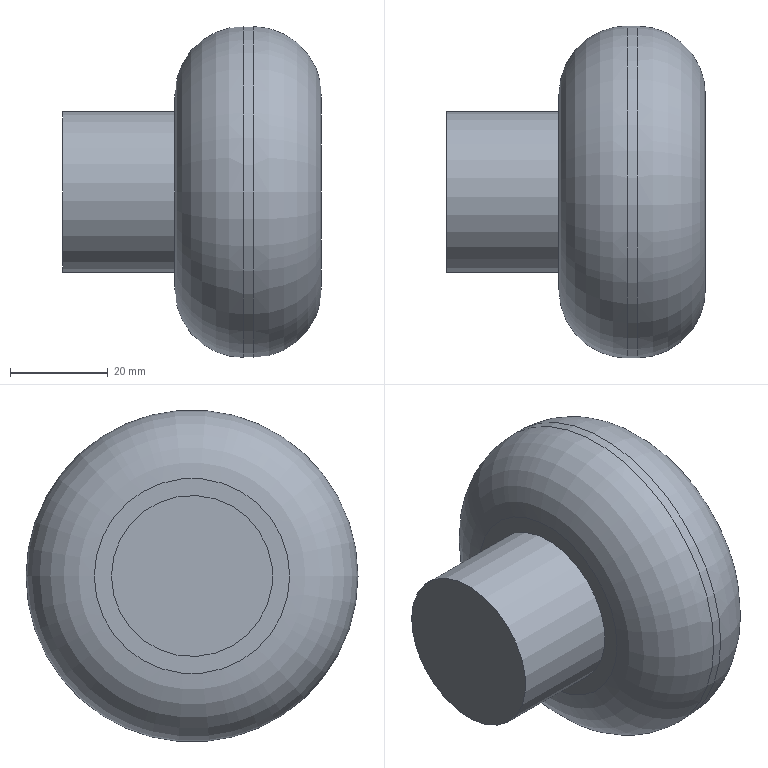Part | STEP file | CMT7E v7 | 1 solid | 7 faces | box 53 x 68 x 68 mm | volume 112304 mm3 | plane 3 | cylinder 2 | torus 2 | commonest cylinder face diameters 33 x1 68 x1
STEP:
#1=CARTESIAN_POINT('',(0.,0.,0.));
#2=DIRECTION('',(0.,0.,1.));
#3=DIRECTION('',(1.,0.,0.));
#4=AXIS2_PLACEMENT_3D('',#1,#2,#3);
#5=CARTESIAN_POINT('',(95.,16.49,-190.));
#6=VERTEX_POINT('',#5);
#7=CARTESIAN_POINT('',(95.,-0.01,-190.));
#8=DIRECTION('',(-1.,0.,0.));
#9=DIRECTION('',(0.,1.,0.));
#10=AXIS2_PLACEMENT_3D('',#7,#8,#9);
#11=CIRCLE('',#10,16.5);
#12=CARTESIAN_POINT('',(95.,-0.01,-190.));
#13=DIRECTION('',(-1.,0.,0.));
#14=DIRECTION('',(0.,1.,0.));
#15=AXIS2_PLACEMENT_3D('',#12,#13,#14);
#16=PLANE('',#15);
#17=CARTESIAN_POINT('',(0.,0.));
#18=DIRECTION('',(1.,0.));
#19=AXIS2_PLACEMENT_2D('',#17,#18);
#20=CIRCLE('',#19,16.5);
#21=(GEOMETRIC_REPRESENTATION_CONTEXT(2)PARAMETRIC_REPRESENTATION_CONTEXT()REPRESENTATION_CONTEXT('',''));
#22=DEFINITIONAL_REPRESENTATION('',(#20),#21);
#23=PCURVE('',#16,#22);
#24=CARTESIAN_POINT('',(95.,-0.01,-190.));
#25=DIRECTION('',(-1.,0.,0.));
#26=DIRECTION('',(0.,1.,0.));
#27=AXIS2_PLACEMENT_3D('',#24,#25,#26);
#28=CYLINDRICAL_SURFACE('',#27,16.5);
#29=CARTESIAN_POINT('',(0.,0.));
#30=DIRECTION('',(1.,0.));
#31=VECTOR('',#30,1.);
#32=LINE('',#29,#31);
#33=(GEOMETRIC_REPRESENTATION_CONTEXT(2)PARAMETRIC_REPRESENTATION_CONTEXT()REPRESENTATION_CONTEXT('',''));
#34=DEFINITIONAL_REPRESENTATION('',(#32),#33);
#35=PCURVE('',#28,#34);
#36=SURFACE_CURVE('',#11,(#23,#35),.PCURVE_S1.);
#37=EDGE_CURVE('',#6,#6,#36,.T.);
#38=ORIENTED_EDGE('',*,*,#37,.T.);
#39=EDGE_LOOP('',(#38));
#40=FACE_BOUND('',#39,.T.);
#41=ADVANCED_FACE('',(#40),#16,.T.);
#42=ORIENTED_EDGE('',*,*,#37,.F.);
#43=CARTESIAN_POINT('',(118.,16.49,-190.));
#44=VERTEX_POINT('',#43);
#45=CARTESIAN_POINT('',(118.,16.49,-190.));
#46=CARTESIAN_POINT('',(95.,16.49,-190.));
#47=B_SPLINE_CURVE_WITH_KNOTS('',1,(#45,#46),.UNSPECIFIED.,.F.,.F.,(2,2),(-23.,0.),.PIECEWISE_BEZIER_KNOTS.);
#48=CARTESIAN_POINT('',(0.,0.));
#49=DIRECTION('',(0.,1.));
#50=VECTOR('',#49,1.);
#51=LINE('',#48,#50);
#52=(GEOMETRIC_REPRESENTATION_CONTEXT(2)PARAMETRIC_REPRESENTATION_CONTEXT()REPRESENTATION_CONTEXT('',''));
#53=DEFINITIONAL_REPRESENTATION('',(#51),#52);
#54=PCURVE('',#28,#53);
#55=CARTESIAN_POINT('',(6.283,0.));
#56=DIRECTION('',(0.,1.));
#57=VECTOR('',#56,1.);
#58=LINE('',#55,#57);
#59=(GEOMETRIC_REPRESENTATION_CONTEXT(2)PARAMETRIC_REPRESENTATION_CONTEXT()REPRESENTATION_CONTEXT('',''));
#60=DEFINITIONAL_REPRESENTATION('',(#58),#59);
#61=PCURVE('',#28,#60);
#62=SEAM_CURVE('',#47,(#54,#61),.PCURVE_S1.);
#63=EDGE_CURVE('',#44,#6,#62,.T.);
#64=ORIENTED_EDGE('',*,*,#63,.F.);
#65=CARTESIAN_POINT('',(118.,-0.01,-190.));
#66=DIRECTION('',(-1.,0.,0.));
#67=DIRECTION('',(0.,1.,0.));
#68=AXIS2_PLACEMENT_3D('',#65,#66,#67);
#69=CIRCLE('',#68,16.5);
#70=CARTESIAN_POINT('',(0.,-23.));
#71=DIRECTION('',(1.,0.));
#72=VECTOR('',#71,1.);
#73=LINE('',#70,#72);
#74=(GEOMETRIC_REPRESENTATION_CONTEXT(2)PARAMETRIC_REPRESENTATION_CONTEXT()REPRESENTATION_CONTEXT('',''));
#75=DEFINITIONAL_REPRESENTATION('',(#73),#74);
#76=PCURVE('',#28,#75);
#77=CARTESIAN_POINT('',(118.,-0.01,-190.));
#78=DIRECTION('',(-1.,0.,0.));
#79=DIRECTION('',(0.,1.,0.));
#80=AXIS2_PLACEMENT_3D('',#77,#78,#79);
#81=PLANE('',#80);
#82=CARTESIAN_POINT('',(0.,0.));
#83=DIRECTION('',(1.,0.));
#84=AXIS2_PLACEMENT_2D('',#82,#83);
#85=CIRCLE('',#84,16.5);
#86=(GEOMETRIC_REPRESENTATION_CONTEXT(2)PARAMETRIC_REPRESENTATION_CONTEXT()REPRESENTATION_CONTEXT('',''));
#87=DEFINITIONAL_REPRESENTATION('',(#85),#86);
#88=PCURVE('',#81,#87);
#89=SURFACE_CURVE('',#69,(#76,#88),.PCURVE_S1.);
#90=EDGE_CURVE('',#44,#44,#89,.T.);
#91=ORIENTED_EDGE('',*,*,#90,.T.);
#92=ORIENTED_EDGE('',*,*,#63,.T.);
#93=EDGE_LOOP('',(#42,#64,#91,#92));
#94=FACE_BOUND('',#93,.T.);
#95=ADVANCED_FACE('',(#94),#28,.T.);
#96=CARTESIAN_POINT('',(148.,19.99,-190.));
#97=VERTEX_POINT('',#96);
#98=CARTESIAN_POINT('',(148.,-0.01,-190.));
#99=DIRECTION('',(1.,0.,0.));
#100=DIRECTION('',(0.,1.,0.));
#101=AXIS2_PLACEMENT_3D('',#98,#99,#100);
#102=CIRCLE('',#101,20.);
#103=CARTESIAN_POINT('',(148.,-0.01,-190.));
#104=DIRECTION('',(-1.,0.,0.));
#105=DIRECTION('',(0.,1.,0.));
#106=AXIS2_PLACEMENT_3D('',#103,#104,#105);
#107=PLANE('',#106);
#108=CARTESIAN_POINT('',(20.,0.));
#109=CARTESIAN_POINT('',(20.,-34.641));
#110=CARTESIAN_POINT('',(-10.,-17.321));
#111=CARTESIAN_POINT('',(-40.,0.));
#112=CARTESIAN_POINT('',(-10.,17.321));
#113=CARTESIAN_POINT('',(20.,34.641));
#114=CARTESIAN_POINT('',(20.,0.));
#115=(BOUNDED_CURVE()B_SPLINE_CURVE(2,(#108,#109,#110,#111,#112,#113,#114),.UNSPECIFIED.,.T.,.F.)B_SPLINE_CURVE_WITH_KNOTS((1,2,2,2,2,1),(-2.094,0.,2.094,4.189,6.283,8.378),.UNSPECIFIED.)CURVE()GEOMETRIC_REPRESENTATION_ITEM()RATIONAL_B_SPLINE_CURVE((1.,0.5,1.,0.5,1.,0.5,1.))REPRESENTATION_ITEM(''));
#116=(GEOMETRIC_REPRESENTATION_CONTEXT(2)PARAMETRIC_REPRESENTATION_CONTEXT()REPRESENTATION_CONTEXT('',''));
#117=DEFINITIONAL_REPRESENTATION('',(#115),#116);
#118=PCURVE('',#107,#117);
#119=CARTESIAN_POINT('',(134.,-0.01,-190.));
#120=DIRECTION('',(1.,0.,0.));
#121=DIRECTION('',(0.,0.,1.));
#122=AXIS2_PLACEMENT_3D('',#119,#120,#121);
#123=TOROIDAL_SURFACE('',#122,20.,14.);
#124=CARTESIAN_POINT('',(-1.571,1.571));
#125=DIRECTION('',(1.,0.));
#126=VECTOR('',#125,1.);
#127=LINE('',#124,#126);
#128=(GEOMETRIC_REPRESENTATION_CONTEXT(2)PARAMETRIC_REPRESENTATION_CONTEXT()REPRESENTATION_CONTEXT('',''));
#129=DEFINITIONAL_REPRESENTATION('',(#127),#128);
#130=PCURVE('',#123,#129);
#131=SURFACE_CURVE('',#102,(#118,#130),.PCURVE_S1.);
#132=EDGE_CURVE('',#97,#97,#131,.T.);
#133=ORIENTED_EDGE('',*,*,#132,.T.);
#134=EDGE_LOOP('',(#133));
#135=FACE_BOUND('',#134,.T.);
#136=ADVANCED_FACE('',(#135),#107,.F.);
#137=CARTESIAN_POINT('',(134.,33.99,-190.));
#138=VERTEX_POINT('',#137);
#139=CARTESIAN_POINT('',(134.,-0.01,-190.));
#140=DIRECTION('',(-1.,0.,0.));
#141=DIRECTION('',(0.,1.,0.));
#142=AXIS2_PLACEMENT_3D('',#139,#140,#141);
#143=CIRCLE('',#142,34.);
#144=CARTESIAN_POINT('',(4.712,0.));
#145=DIRECTION('',(-1.,0.));
#146=VECTOR('',#145,1.);
#147=LINE('',#144,#146);
#148=(GEOMETRIC_REPRESENTATION_CONTEXT(2)PARAMETRIC_REPRESENTATION_CONTEXT()REPRESENTATION_CONTEXT('',''));
#149=DEFINITIONAL_REPRESENTATION('',(#147),#148);
#150=PCURVE('',#123,#149);
#151=CARTESIAN_POINT('',(118.,-0.01,-190.));
#152=DIRECTION('',(-1.,0.,0.));
#153=DIRECTION('',(0.,1.,0.));
#154=AXIS2_PLACEMENT_3D('',#151,#152,#153);
#155=CYLINDRICAL_SURFACE('',#154,34.);
#156=CARTESIAN_POINT('',(0.,-16.));
#157=DIRECTION('',(1.,0.));
#158=VECTOR('',#157,1.);
#159=LINE('',#156,#158);
#160=(GEOMETRIC_REPRESENTATION_CONTEXT(2)PARAMETRIC_REPRESENTATION_CONTEXT()REPRESENTATION_CONTEXT('',''));
#161=DEFINITIONAL_REPRESENTATION('',(#159),#160);
#162=PCURVE('',#155,#161);
#163=SURFACE_CURVE('',#143,(#150,#162),.PCURVE_S1.);
#164=EDGE_CURVE('',#138,#138,#163,.T.);
#165=ORIENTED_EDGE('',*,*,#164,.F.);
#166=CARTESIAN_POINT('',(134.,33.99,-190.));
#167=CARTESIAN_POINT('',(137.743,33.99,-190.));
#168=CARTESIAN_POINT('',(141.388,32.8,-190.));
#169=CARTESIAN_POINT('',(144.527,30.517,-190.));
#170=CARTESIAN_POINT('',(146.81,27.378,-190.));
#171=CARTESIAN_POINT('',(148.,23.733,-190.));
#172=CARTESIAN_POINT('',(148.,19.99,-190.));
#173=(BOUNDED_CURVE()B_SPLINE_CURVE(6,(#166,#167,#168,#169,#170,#171,#172),.UNSPECIFIED.,.F.,.F.)B_SPLINE_CURVE_WITH_KNOTS((7,7),(0.,1.571),.PIECEWISE_BEZIER_KNOTS.)CURVE()GEOMETRIC_REPRESENTATION_ITEM()RATIONAL_B_SPLINE_CURVE((1.031,1.01,0.9979,0.994,0.9979,1.01,1.031))REPRESENTATION_ITEM(''));
#174=CARTESIAN_POINT('',(4.712,0.));
#175=DIRECTION('',(0.,1.));
#176=VECTOR('',#175,1.);
#177=LINE('',#174,#176);
#178=(GEOMETRIC_REPRESENTATION_CONTEXT(2)PARAMETRIC_REPRESENTATION_CONTEXT()REPRESENTATION_CONTEXT('',''));
#179=DEFINITIONAL_REPRESENTATION('',(#177),#178);
#180=PCURVE('',#123,#179);
#181=CARTESIAN_POINT('',(-1.571,0.));
#182=DIRECTION('',(0.,1.));
#183=VECTOR('',#182,1.);
#184=LINE('',#181,#183);
#185=(GEOMETRIC_REPRESENTATION_CONTEXT(2)PARAMETRIC_REPRESENTATION_CONTEXT()REPRESENTATION_CONTEXT('',''));
#186=DEFINITIONAL_REPRESENTATION('',(#184),#185);
#187=PCURVE('',#123,#186);
#188=SEAM_CURVE('',#173,(#180,#187),.PCURVE_S1.);
#189=EDGE_CURVE('',#138,#97,#188,.T.);
#190=ORIENTED_EDGE('',*,*,#189,.T.);
#191=ORIENTED_EDGE('',*,*,#132,.F.);
#192=ORIENTED_EDGE('',*,*,#189,.F.);
#193=EDGE_LOOP('',(#165,#190,#191,#192));
#194=FACE_BOUND('',#193,.T.);
#195=ADVANCED_FACE('',(#194),#123,.T.);
#196=ORIENTED_EDGE('',*,*,#90,.F.);
#197=EDGE_LOOP('',(#196));
#198=FACE_BOUND('',#197,.T.);
#199=CARTESIAN_POINT('',(118.,19.99,-190.));
#200=VERTEX_POINT('',#199);
#201=CARTESIAN_POINT('',(118.,-0.01,-190.));
#202=DIRECTION('',(-1.,0.,0.));
#203=DIRECTION('',(0.,1.,0.));
#204=AXIS2_PLACEMENT_3D('',#201,#202,#203);
#205=CIRCLE('',#204,20.);
#206=CARTESIAN_POINT('',(0.,0.));
#207=DIRECTION('',(1.,0.));
#208=AXIS2_PLACEMENT_2D('',#206,#207);
#209=CIRCLE('',#208,20.);
#210=(GEOMETRIC_REPRESENTATION_CONTEXT(2)PARAMETRIC_REPRESENTATION_CONTEXT()REPRESENTATION_CONTEXT('',''));
#211=DEFINITIONAL_REPRESENTATION('',(#209),#210);
#212=PCURVE('',#81,#211);
#213=CARTESIAN_POINT('',(132.,-0.01,-190.));
#214=DIRECTION('',(1.,0.,0.));
#215=DIRECTION('',(0.,0.,1.));
#216=AXIS2_PLACEMENT_3D('',#213,#214,#215);
#217=TOROIDAL_SURFACE('',#216,20.,14.);
#218=CARTESIAN_POINT('',(4.712,4.712));
#219=DIRECTION('',(-1.,0.));
#220=VECTOR('',#219,1.);
#221=LINE('',#218,#220);
#222=(GEOMETRIC_REPRESENTATION_CONTEXT(2)PARAMETRIC_REPRESENTATION_CONTEXT()REPRESENTATION_CONTEXT('',''));
#223=DEFINITIONAL_REPRESENTATION('',(#221),#222);
#224=PCURVE('',#217,#223);
#225=SURFACE_CURVE('',#205,(#212,#224),.PCURVE_S1.);
#226=EDGE_CURVE('',#200,#200,#225,.T.);
#227=ORIENTED_EDGE('',*,*,#226,.T.);
#228=EDGE_LOOP('',(#227));
#229=FACE_BOUND('',#228,.T.);
#230=ADVANCED_FACE('',(#198,#229),#81,.T.);
#231=CARTESIAN_POINT('',(132.,33.99,-190.));
#232=VERTEX_POINT('',#231);
#233=CARTESIAN_POINT('',(132.,-0.01,-190.));
#234=DIRECTION('',(1.,0.,0.));
#235=DIRECTION('',(0.,1.,0.));
#236=AXIS2_PLACEMENT_3D('',#233,#234,#235);
#237=CIRCLE('',#236,34.);
#238=CARTESIAN_POINT('',(6.283,-14.));
#239=DIRECTION('',(-1.,0.));
#240=VECTOR('',#239,1.);
#241=LINE('',#238,#240);
#242=(GEOMETRIC_REPRESENTATION_CONTEXT(2)PARAMETRIC_REPRESENTATION_CONTEXT()REPRESENTATION_CONTEXT('',''));
#243=DEFINITIONAL_REPRESENTATION('',(#241),#242);
#244=PCURVE('',#155,#243);
#245=CARTESIAN_POINT('',(-1.571,6.283));
#246=DIRECTION('',(1.,0.));
#247=VECTOR('',#246,1.);
#248=LINE('',#245,#247);
#249=(GEOMETRIC_REPRESENTATION_CONTEXT(2)PARAMETRIC_REPRESENTATION_CONTEXT()REPRESENTATION_CONTEXT('',''));
#250=DEFINITIONAL_REPRESENTATION('',(#248),#249);
#251=PCURVE('',#217,#250);
#252=SURFACE_CURVE('',#237,(#244,#251),.PCURVE_S1.);
#253=EDGE_CURVE('',#232,#232,#252,.T.);
#254=ORIENTED_EDGE('',*,*,#253,.T.);
#255=CARTESIAN_POINT('',(134.,33.99,-190.));
#256=CARTESIAN_POINT('',(132.,33.99,-190.));
#257=B_SPLINE_CURVE_WITH_KNOTS('',1,(#255,#256),.UNSPECIFIED.,.F.,.F.,(2,2),(-16.,-14.),.PIECEWISE_BEZIER_KNOTS.);
#258=CARTESIAN_POINT('',(0.,0.));
#259=DIRECTION('',(0.,1.));
#260=VECTOR('',#259,1.);
#261=LINE('',#258,#260);
#262=(GEOMETRIC_REPRESENTATION_CONTEXT(2)PARAMETRIC_REPRESENTATION_CONTEXT()REPRESENTATION_CONTEXT('',''));
#263=DEFINITIONAL_REPRESENTATION('',(#261),#262);
#264=PCURVE('',#155,#263);
#265=CARTESIAN_POINT('',(6.283,0.));
#266=DIRECTION('',(0.,1.));
#267=VECTOR('',#266,1.);
#268=LINE('',#265,#267);
#269=(GEOMETRIC_REPRESENTATION_CONTEXT(2)PARAMETRIC_REPRESENTATION_CONTEXT()REPRESENTATION_CONTEXT('',''));
#270=DEFINITIONAL_REPRESENTATION('',(#268),#269);
#271=PCURVE('',#155,#270);
#272=SEAM_CURVE('',#257,(#264,#271),.PCURVE_S1.);
#273=EDGE_CURVE('',#138,#232,#272,.T.);
#274=ORIENTED_EDGE('',*,*,#273,.F.);
#275=ORIENTED_EDGE('',*,*,#164,.T.);
#276=ORIENTED_EDGE('',*,*,#273,.T.);
#277=EDGE_LOOP('',(#254,#274,#275,#276));
#278=FACE_BOUND('',#277,.T.);
#279=ADVANCED_FACE('',(#278),#155,.T.);
#280=ORIENTED_EDGE('',*,*,#226,.F.);
#281=CARTESIAN_POINT('',(118.,19.99,-190.));
#282=CARTESIAN_POINT('',(118.,23.733,-190.));
#283=CARTESIAN_POINT('',(119.19,27.378,-190.));
#284=CARTESIAN_POINT('',(121.473,30.517,-190.));
#285=CARTESIAN_POINT('',(124.612,32.8,-190.));
#286=CARTESIAN_POINT('',(128.257,33.99,-190.));
#287=CARTESIAN_POINT('',(132.,33.99,-190.));
#288=(BOUNDED_CURVE()B_SPLINE_CURVE(6,(#281,#282,#283,#284,#285,#286,#287),.UNSPECIFIED.,.F.,.F.)B_SPLINE_CURVE_WITH_KNOTS((7,7),(4.712,6.283),.PIECEWISE_BEZIER_KNOTS.)CURVE()GEOMETRIC_REPRESENTATION_ITEM()RATIONAL_B_SPLINE_CURVE((1.031,1.01,0.9979,0.994,0.9979,1.01,1.031))REPRESENTATION_ITEM(''));
#289=CARTESIAN_POINT('',(4.712,0.));
#290=DIRECTION('',(0.,1.));
#291=VECTOR('',#290,1.);
#292=LINE('',#289,#291);
#293=(GEOMETRIC_REPRESENTATION_CONTEXT(2)PARAMETRIC_REPRESENTATION_CONTEXT()REPRESENTATION_CONTEXT('',''));
#294=DEFINITIONAL_REPRESENTATION('',(#292),#293);
#295=PCURVE('',#217,#294);
#296=CARTESIAN_POINT('',(-1.571,0.));
#297=DIRECTION('',(0.,1.));
#298=VECTOR('',#297,1.);
#299=LINE('',#296,#298);
#300=(GEOMETRIC_REPRESENTATION_CONTEXT(2)PARAMETRIC_REPRESENTATION_CONTEXT()REPRESENTATION_CONTEXT('',''));
#301=DEFINITIONAL_REPRESENTATION('',(#299),#300);
#302=PCURVE('',#217,#301);
#303=SEAM_CURVE('',#288,(#295,#302),.PCURVE_S1.);
#304=EDGE_CURVE('',#200,#232,#303,.T.);
#305=ORIENTED_EDGE('',*,*,#304,.T.);
#306=ORIENTED_EDGE('',*,*,#253,.F.);
#307=ORIENTED_EDGE('',*,*,#304,.F.);
#308=EDGE_LOOP('',(#280,#305,#306,#307));
#309=FACE_BOUND('',#308,.T.);
#310=ADVANCED_FACE('',(#309),#217,.T.);
#311=CLOSED_SHELL('',(#41,#95,#136,#195,#230,#279,#310));
#312=MANIFOLD_SOLID_BREP('',#311);
#313=(LENGTH_UNIT()NAMED_UNIT(*)SI_UNIT(.MILLI.,.METRE.));
#314=UNCERTAINTY_MEASURE_WITH_UNIT(LENGTH_MEASURE(0.000002),#313,'','');
#315=(NAMED_UNIT(*)PLANE_ANGLE_UNIT()SI_UNIT($,.RADIAN.));
#316=(NAMED_UNIT(*)SI_UNIT($,.STERADIAN.)SOLID_ANGLE_UNIT());
#317=(GEOMETRIC_REPRESENTATION_CONTEXT(3)GLOBAL_UNCERTAINTY_ASSIGNED_CONTEXT((#314))GLOBAL_UNIT_ASSIGNED_CONTEXT((#313,#315,#316))REPRESENTATION_CONTEXT('',''));
#318=ADVANCED_BREP_SHAPE_REPRESENTATION('',(#4,#312),#317);